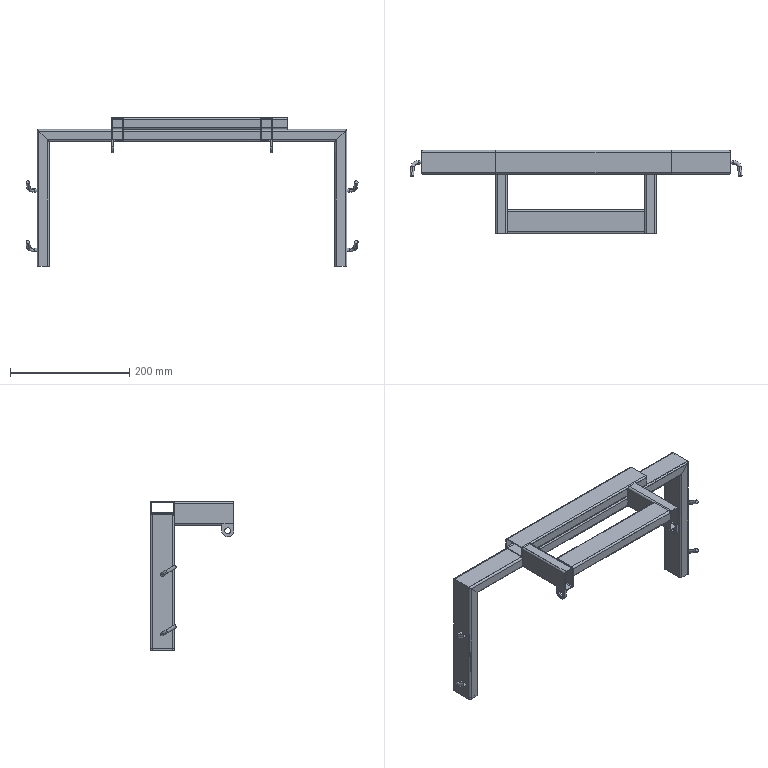Part | SolidWorks | features WeldCornerFeat 4, ICE 3, WeldMemberFeat 3, 3DProfileFeature 2, LPattern 1, MirrorPattern 1, Sweep 1, WeldmentFeature 1 | 9 solids | 175 faces | box 557.288 x 140 x 250 mm | volume 285263 mm3 | plane 88 | cylinder 79 | torus 8 | commonest cylinder face diameters 6 x44 3 x28 10 x4 20 x3